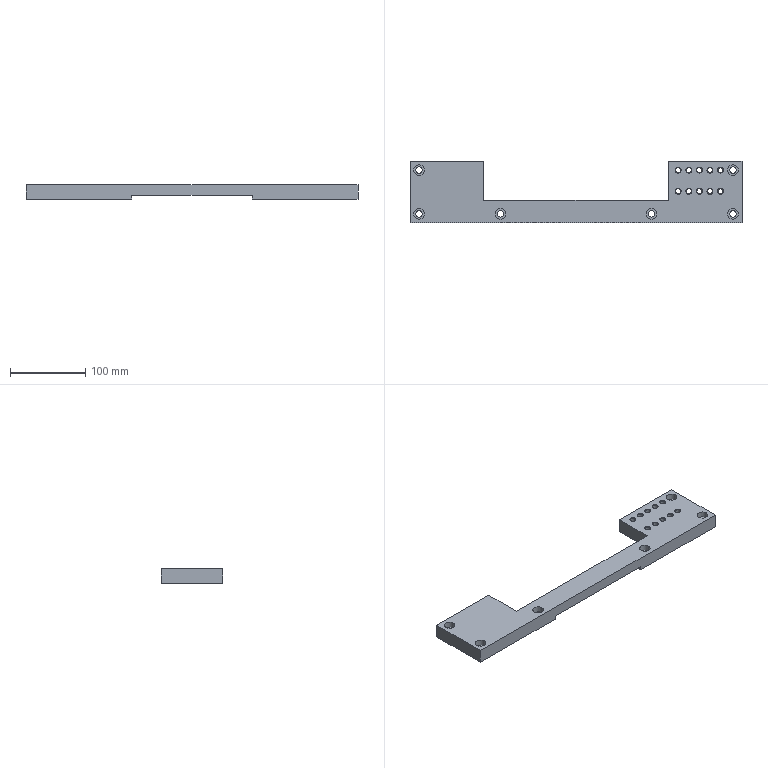Part | STEP file | Tube necking machine_id686_x_t | 1 solid | 62 faces | box 440 x 82 x 19 mm | volume 401344 mm3 | cylinder 22 | cone 20 | plane 20 | commonest cylinder face diameters 6.8 x10 8.5 x6 14 x6